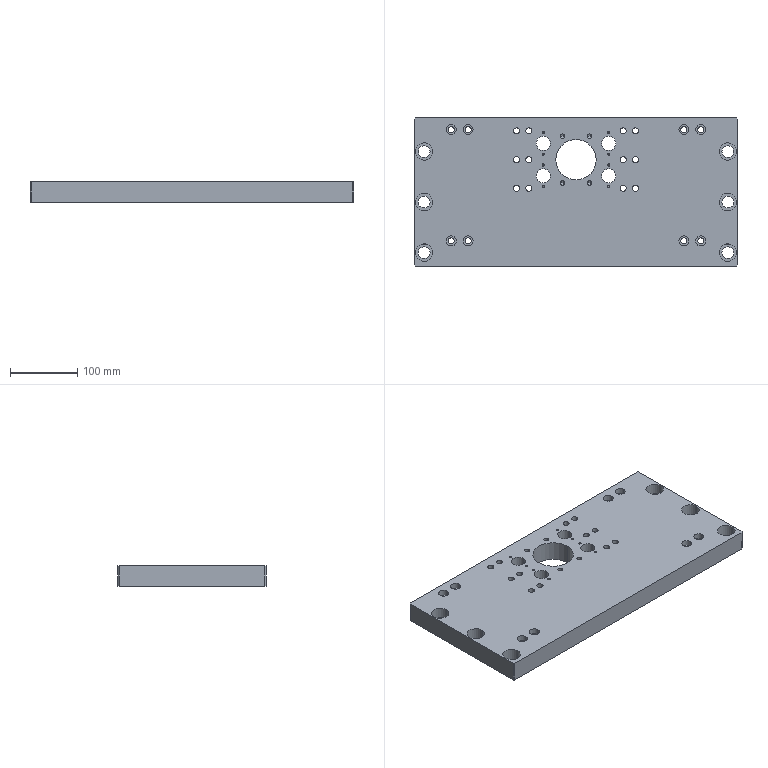Part | SolidWorks | features HoleWzd 5, Chamfer 1, Cut 1, Extrusion 1, ICE 1, MirrorPattern 1 | 1 solid | 198 faces | box 480 x 220 x 30 mm | volume 2905739 mm3 | cylinder 138 | plane 36 | cone 24 | commonest cylinder face diameters 9 x40 15 x40 3.3 x16 17.5 x12 26 x12 6.8 x8